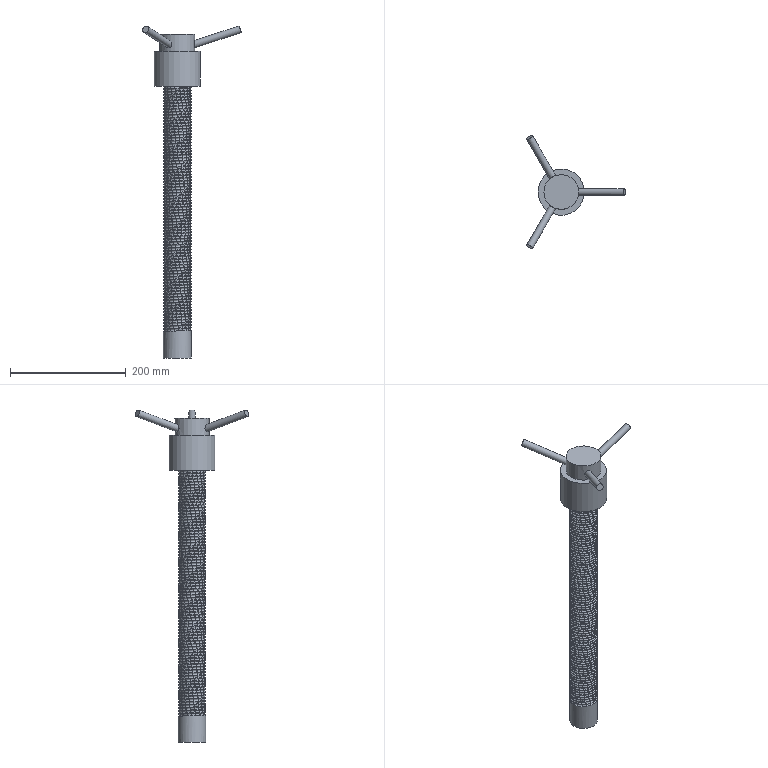Part | NX | features CYLINDER 4, DATUM_CSYS 3, DATUM_PLANE 3, EXTRACT_BODY 2, SKETCH 2, EXTRUDE 1, HELIX 1, Pattern Geometry 1, SWP104 1, UNITE 1 | 1 solid | 1644 faces | box 170.632 x 195.599 x 574.025 mm | volume 1187331 mm3 | torus 1544 | cylinder 91 | plane 9 | commonest cylinder face diameters 48 x86 12 x3 60 x1 80 x1